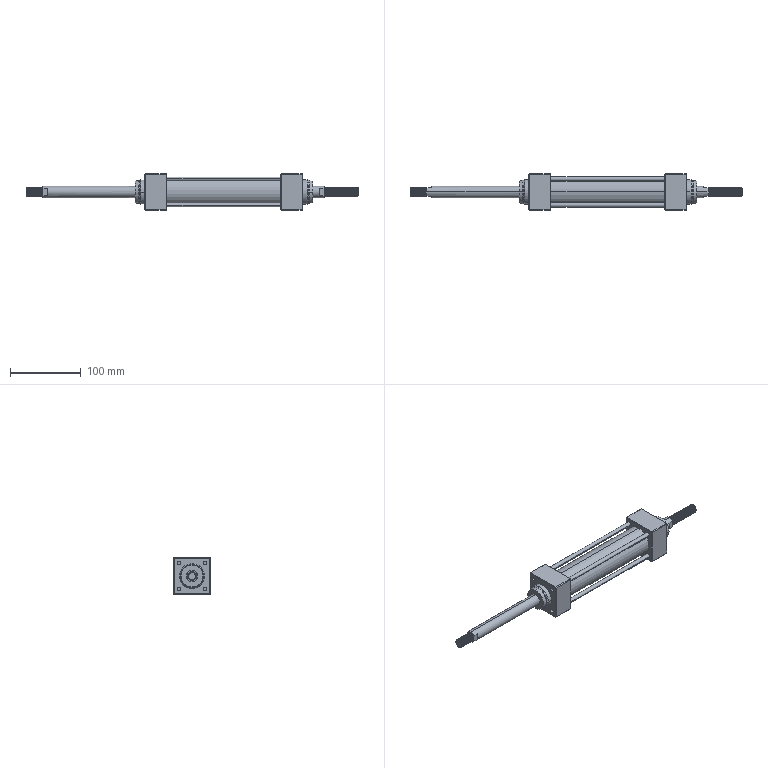Part | STEP file | PN_0017 | 1 solid | 247 faces | box 469 x 52 x 52 mm | volume 443699 mm3 | cylinder 149 | plane 60 | spline 30 | torus 4 | cone 4 | commonest cylinder face diameters 12 x111 5 x16 6 x8 16 x4 33 x4 35 x4